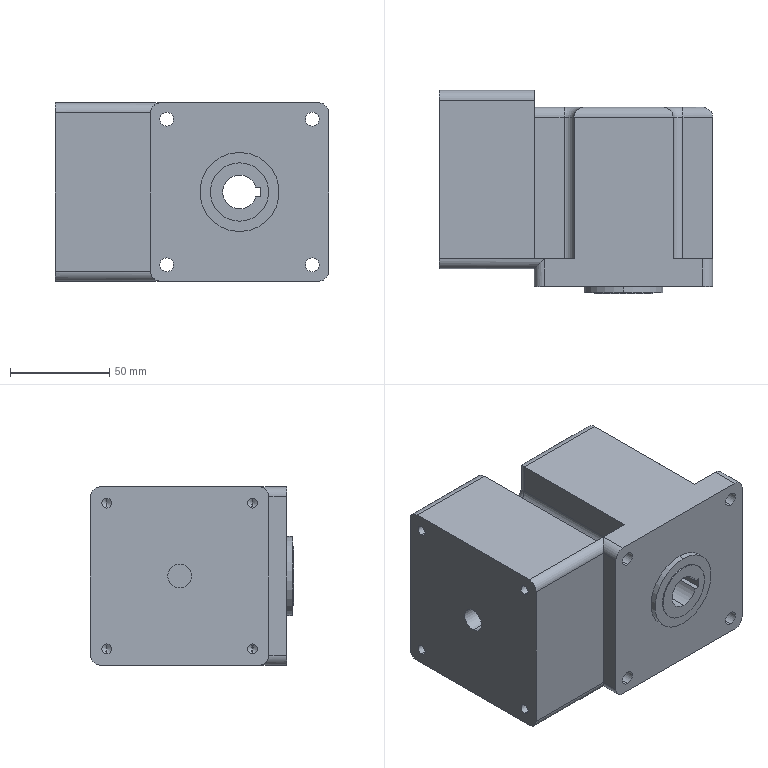Part | SolidWorks | features ICE 10, Fillet 6, CirPattern 3, HoleWzd 2, Chamfer 1, Extrusion 1 | 1 solid | 90 faces | box 138 x 102.5 x 90 mm | volume 973756 mm3 | cylinder 48 | plane 30 | cone 8 | torus 4 | commonest cylinder face diameters 10 x22 5 x8 7 x8 17 x3 12 x2 29.5 x2